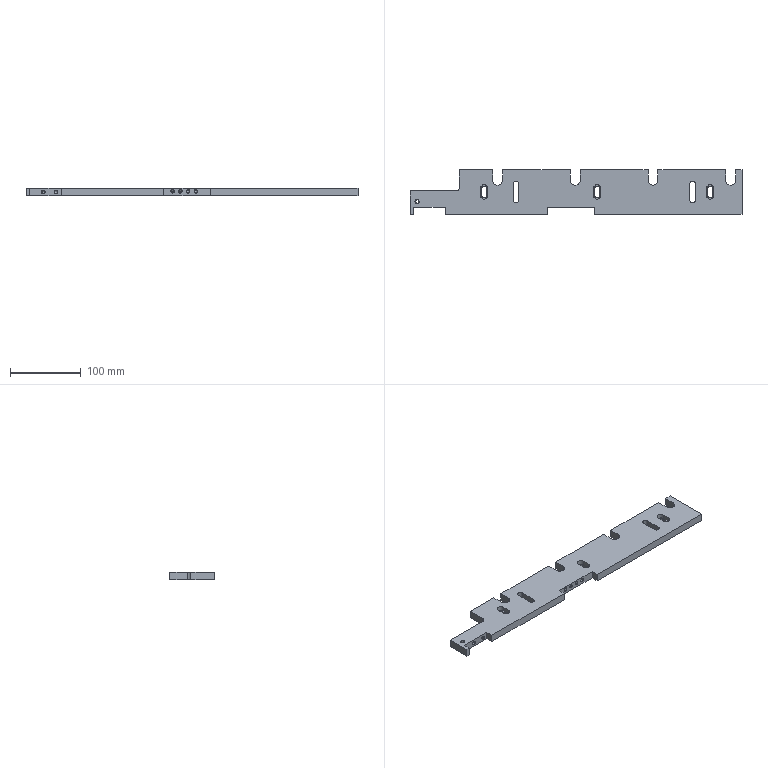Part | STEP file | Tube feed_id562_x_t | 1 solid | 89 faces | box 470 x 63 x 11 mm | volume 265889 mm3 | plane 47 | cylinder 28 | cone 14 | commonest cylinder face diameters 4.2 x6 6.8 x6 10.5 x6 8 x4 14 x4 5 x1